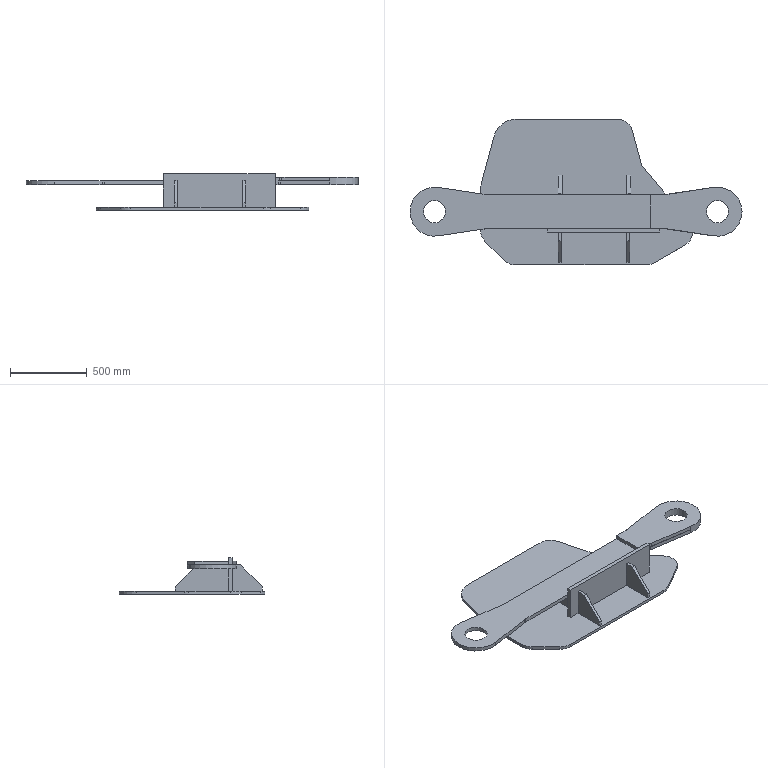Part | NX | features 后连杆右 2 | 1 solid | 72 faces | box 2165 x 950 x 239.704 mm | volume 42809177 mm3 | plane 55 | cylinder 17 | commonest cylinder face diameters 200 x12 145 x2 320 x2 300 x1